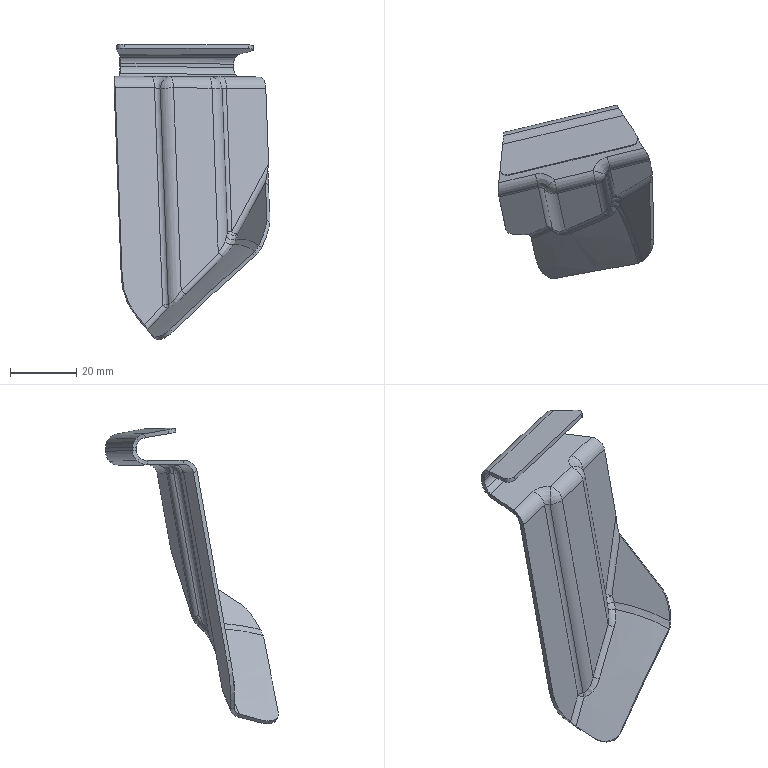Part | 1 solid | 98 faces | box 47.154 x 52.368 x 89.463 mm | volume 6233 mm3 | spline 55 | cylinder 24 | plane 10 | sphere 8 | other 1 | commonest cylinder face diameters 6 x12 8.4 x9 3.6 x3